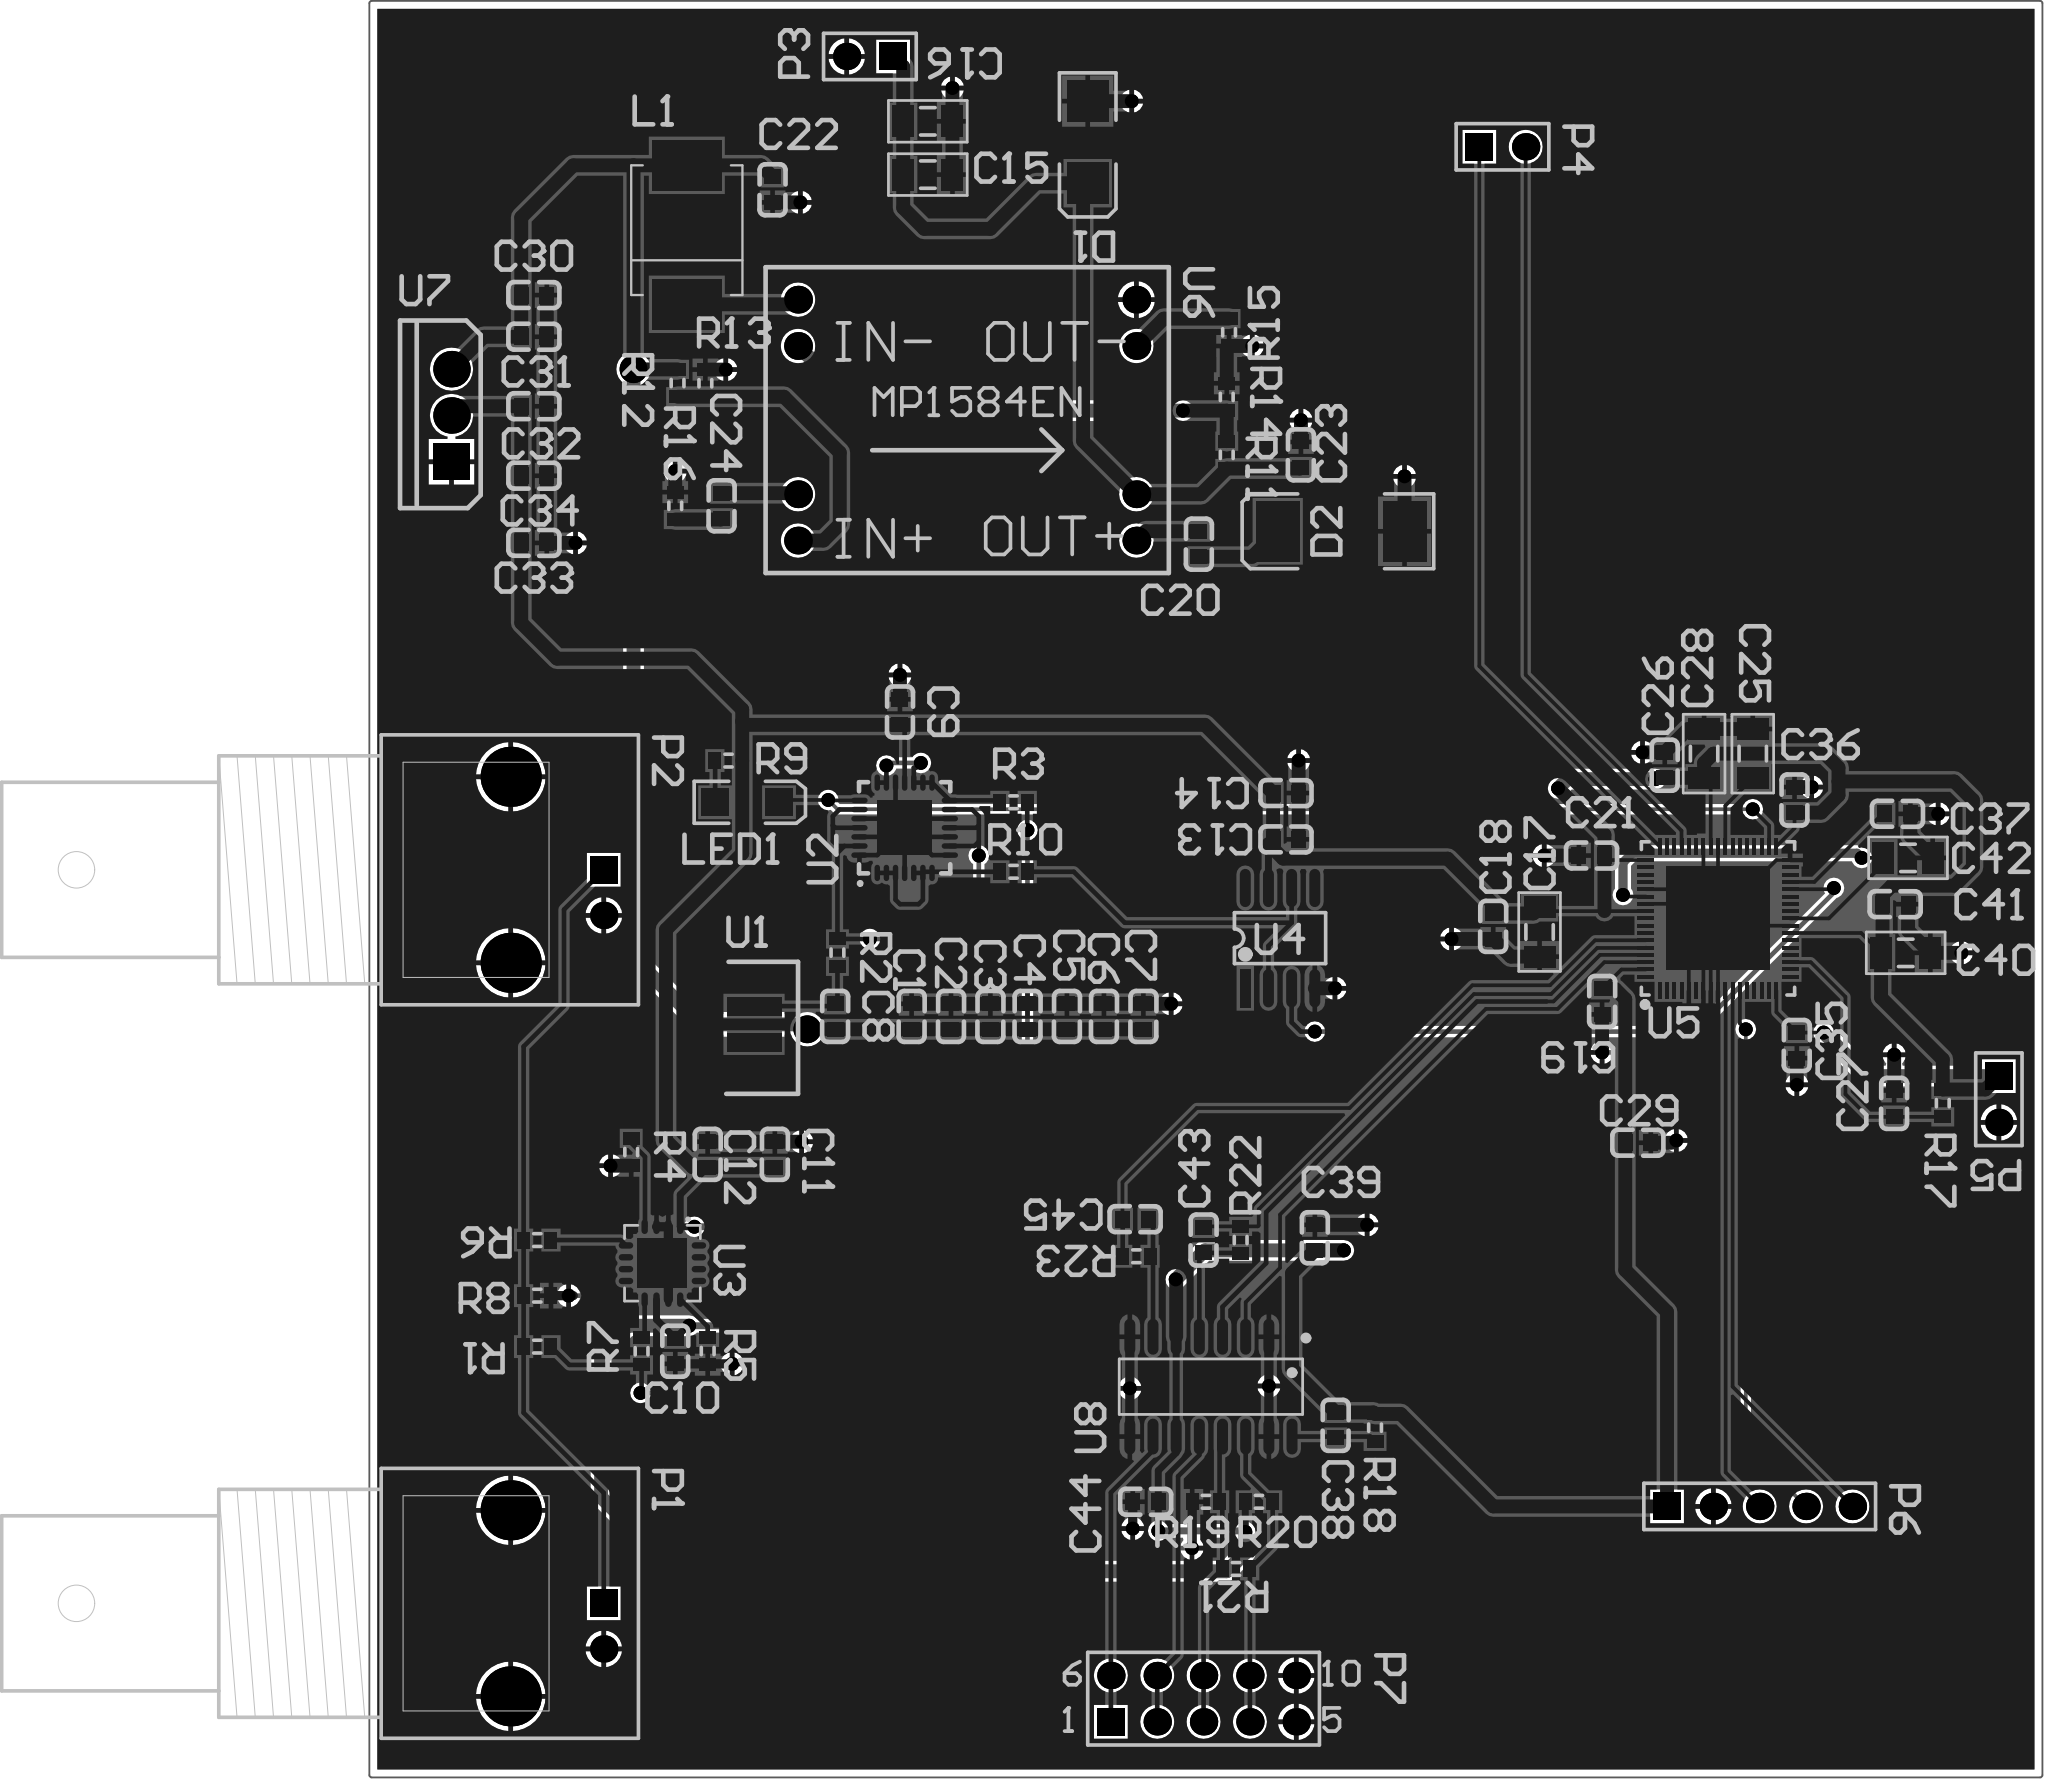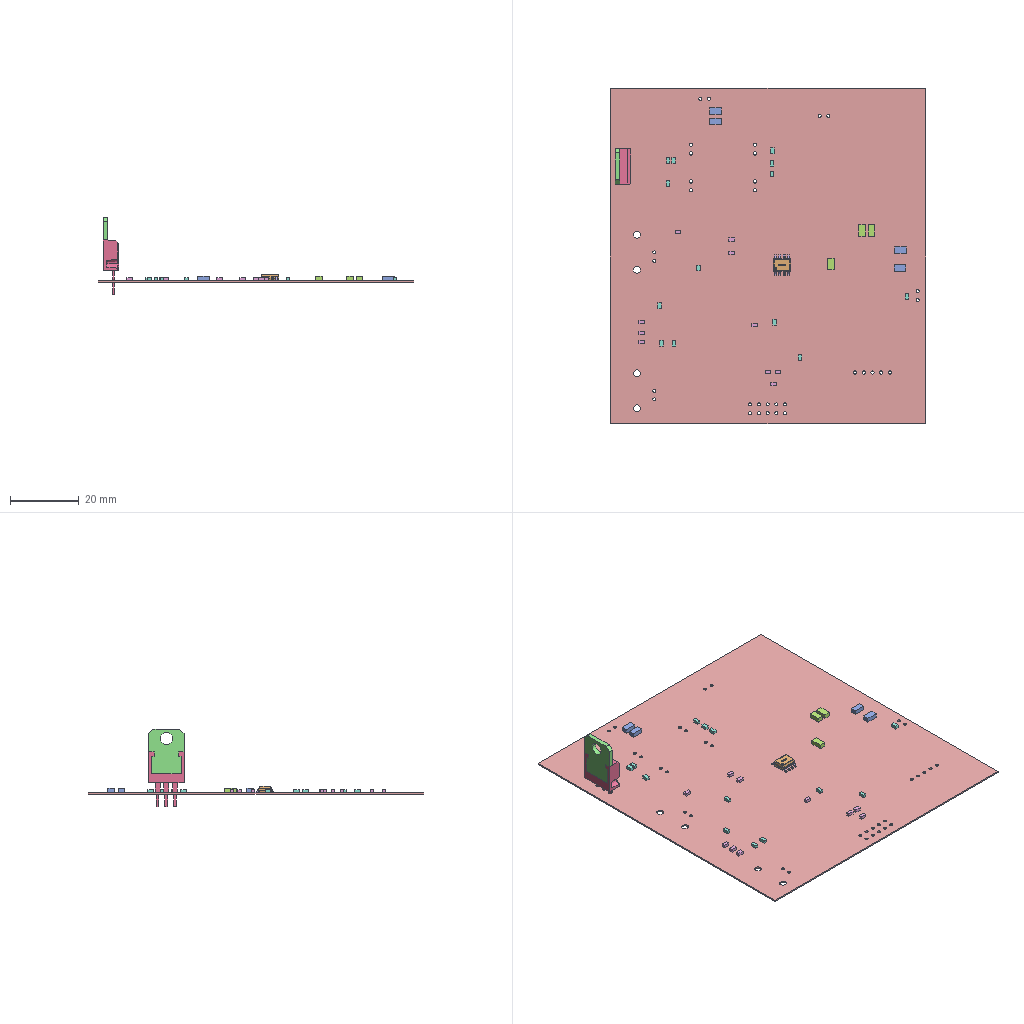Circuit board layout | Altium Designer | box 91.7 x 97.4 x 22.5 mm
Layer stack:
# Altium Designer layer stack of  (unit mm; dielectric type: 0 none, 1 core, 2 prepreg, 3 surface material)
index,name,kind,layer,copper_thickness_mm,dielectric_type,dielectric_thickness_mm,dielectric_material,dielectric_constant
0,Top Paste,other,,,,,,
1,Top Overlay,other,,,,,,
2,Top Solder,dielectric,,,3,0.0102,Solder Resist,3.5
3,Top Layer,copper,Top Layer,0.0356,,,,
4,Dielectric 1,dielectric,,,0,0.32,FR-4,4.8
5,Bottom Layer,copper,Bottom Layer,0.0356,,,,
6,Bottom Solder,dielectric,,,3,0.0102,Solder Resist,3.5
7,Bottom Overlay,other,,,,,,
8,Bottom Paste,other,,,,,,
# drill layer pairs: low layer,high layer
drill_pair,Top Layer,Bottom Layer
Part placement:
Designator,Comment,Layer,Footprint,Center-X(mm),Center-Y(mm),Rotation
C1,10UF,TopLayer,C0603,54.991,71.436,270
C2,10UF,TopLayer,C0603,57.15,71.436,270
C3,10UF,TopLayer,C0603,59.309,71.436,270
C4,10UF,TopLayer,C0603,61.344,71.436,270
C5,10UF,TopLayer,C0603,63.503,71.436,270
C6,0.1UF,TopLayer,C0603,65.532,71.436,270
C7,10UF,TopLayer,C0603,67.694,71.436,270
C8,100PF,TopLayer,C0603,50.797,71.436,270
C9,10UF,TopLayer,C0603,54.353,88.13,270
C10,0.1UF,TopLayer,C0603,42.04,53.094,90
C11,0.1UF,TopLayer,C0603,47.495,63.873,270
C12,10UF,TopLayer,C0603,43.812,63.873,270
C13,0.1UF,TopLayer,C0603,75.503,81.153,180
C14,10UF,TopLayer,C0603,75.503,83.693,180
C15,10UF/50V,TopLayer,C1206,55.88,117.602,180
C16,10UF/50V,TopLayer,C1206,55.88,120.523,180
C17,1UF/16V,TopLayer,C1206,89.408,76.073,90
C18,0.1UF,TopLayer,C0603,86.868,76.389,90
C19,0.1UF,TopLayer,C0603,92.834,72.255,270
C20,0.1UF,TopLayer,C0603,70.739,97.347,90
C21,0.1UF,TopLayer,C0603,92.264,80.264,0
C22,22UF,TopLayer,C0603,47.371,116.778,90
C23,10UF,TopLayer,C0603,76.33,102.243,90
C24,150PF,TopLayer,C0603,44.574,99.433,270
C25,1UF/16V,TopLayer,C1206,101.092,85.852,270
C26,0.1UF,TopLayer,C0603,96.269,85.225,90
C27,10nf,TopLayer,C0603,108.842,66.683,90
C28,1UF/16V,TopLayer,C1206,98.425,85.852,90
C29,0.1UF,TopLayer,C0603,94.804,64.516,360
C30,10UF,TopLayer,C0603,34.298,110.995,360
C31,0.1UF,TopLayer,C0603,34.298,108.709,360
C32,10UF,TopLayer,C0603,34.298,104.899,360
C33,1UF,TopLayer,C0603,34.298,97.406,360
C34,0.1UF,TopLayer,C0603,34.298,101.089,360
C35,0.1UF,TopLayer,C0603,103.508,69.858,90
C36,0.1UF,TopLayer,C0603,103.381,83.32,90
C37,0.1UF,TopLayer,C0603,109.031,82.55,360
C38,12PF,TopLayer,C0603,78.235,49.03,90
C39,0.1UF,TopLayer,C0603,77.092,59.317,90
C40,1UF/16V,TopLayer,C1206,109.474,74.93,360
C41,0.1UF,TopLayer,C0603,108.904,77.597,360
C42,1UF/16V,TopLayer,C1206,109.601,80.137,360
C43,12PF,TopLayer,C0603,70.99,59.174,270
C44,01.UF,TopLayer,C0603,67.81,44.834,180
C45,12PF,TopLayer,C0603,67.248,60.325,360
D1,D Schottky,TopLayer,SMB,64.643,119.38,270
D2,S320,TopLayer,SMC,78.532,98.044,180
L1,22UH,TopLayer,DIODE_SMC,42.672,114.3,90
LED1,LED2,TopLayer,3.2X1.6X1.1,45.974,83.185,360
P1,BNC,TopLayer,BNC_RA_CON,35.57,39.263,360
P2,BNC,TopLayer,BNC_RA_CON,35.57,79.482,360
P3,Header 2,TopLayer,HDR1X2,52.705,124.079,180
P4,Header 2,TopLayer,HDR1X2,87.376,119.126,360
P5,Header 2,TopLayer,HDR1X2,114.581,66.902,270
P6,Header 5,TopLayer,HDR1X5,101.473,44.577,360
P7,Header 5X2A,TopLayer,HDR2X5_CEN,70.993,34.036,360
R1,N/A,TopLayer,J1-0603,34.477,53.34,180
R2,0.1,TopLayer,J1-0603,50.927,74.942,270
R3,33,TopLayer,J1-0603,60.579,83.185,0
R4,4.7K,TopLayer,J1-0603,39.624,64.008,270
R5,4.7K,TopLayer,J1-0603,43.815,53.098,90
R6,33,TopLayer,J1-0603,34.477,59.182,180
R7,0,TopLayer,J1-0603,40.192,53.086,90
R8,510,TopLayer,J1-0603,34.477,56.134,360
R9,10K,TopLayer,J1-0603,44.958,85.471,0
R10,33,TopLayer,J1-0603,60.579,79.375,360
R11,100K,TopLayer,J1-0603,72.263,102.235,270
R12,300K,TopLayer,J1-0603,42.164,106.172,270
R13,39K,TopLayer,J1-0603,43.688,106.16,90
R14,25K,TopLayer,J1-0603,72.263,105.41,270
R15,100K,TopLayer,J1-0603,72.39,108.954,90
R16,100K,TopLayer,J1-0603,42.037,99.441,270
R17,10K,TopLayer,J1-0603,111.506,66.687,90
R18,820,TopLayer,J1-0603,80.391,48.895,270
R19,510,TopLayer,J1-0603,71.12,44.831,360
R20,510,TopLayer,J1-0603,74.029,44.831,360
R21,120,TopLayer,J1-0603,72.771,41.148,180
R22,10K,TopLayer,J1-0603,73.025,59.182,90
R23,820,TopLayer,J1-0603,67.31,58.293,360
U1,Laser diode,TopLayer,激光二极管,46.355,71.009,90
U2,IC-HG,TopLayer,QFN28-5X5,54.61,81.788,90
U3,ISL55111IRZ-T,TopLayer,QFN-16_L4.0-W4.0-P0.65-BL-EP2.6,41.335,57.912,180
U4,OPA335AIDRG4,TopLayer,SOP8,75.184,75.736,90
U5,CY8C3245LTI-163,TopLayer,QFN-68_L8.0-W8.0-P0.40-TL-EP5.7,99.187,76.818,90
U7,LM317,TopLayer,TO220A,29.774,104.394,90
U8,IL3122-3E,TopLayer,SOIC-16_L9.9-W3.9-P1.27-LS6.0-BL,71.396,51.143,180
U6,MP1584ENZ,TopLayer,MP1548EN,58.038,104.14,360
Pad and via stacks:
# Altium Designer via and pad stacks of  (unit mm). Each distinct definition once, with the count of objects using it.
# via: kind,start_layer,end_layer,hole_mm,diameter_mm,mode(0 simple;1 top-mid-bottom;2 full stack),diameter_per_layer,count,example_net
# pad: kind,layer,hole_mm,hole_type(0 round;1 square;2 slot),plating,top_size,top_shape(1 round;2 rect;3 octagon;9 rounded rect),mid_size,bottom_size,mode,footprint,size_per_layer,count,example
pad,Top Layer,0,0,plated,0.8x0.9,2,0.8x0.9,0.8x0.9,0,C0603,,76,C45.2
pad,Top Layer,0,0,plated,0.9x0.7,2,0.9x0.7,0.9x0.7,0,J1-0603,,46,R23.2
pad,Top Layer,0,0,plated,1.7x1.2,2,1.7x1.2,1.7x1.2,0,C1206,,14,C40.2
pad,Top Layer,0,0,plated,0.602x1.971,1,0.602x1.971,0.602x1.971,0,SOIC-16_L9.9-W3.9-P1.27-LS6.0-BL,,16,U8.9
pad,Top Layer,0,0,plated,2.794x3.81,2,2.794x3.81,2.794x3.81,0,DIODE_SMC,,2,L1.1
pad,Top Layer,0,0,plated,0.2x0.9,2,0.2x0.9,0.2x0.9,0,QFN-68_L8.0-W8.0-P0.40-TL-EP5.7,,34,U5.17
pad,Top Layer,0,0,plated,5.7x5.7,2,5.7x5.7,5.7x5.7,0,QFN-68_L8.0-W8.0-P0.40-TL-EP5.7,,1,U5.69
pad,Top Layer,0,0,plated,0.9x0.2,2,0.9x0.2,0.9x0.2,0,QFN-68_L8.0-W8.0-P0.40-TL-EP5.7,,34,U5.18
pad,Top Layer,0,0,plated,2.4x3.3,2,2.4x3.3,2.4x3.3,0,SMC,,2,D2.2
pad,Top Layer,0,0,plated,2.3x2.3,2,2.3x2.3,2.3x2.3,0,SMB,,2,D1.1
pad,Top Layer,0,0,plated,1.5x1.5,2,1.5x1.5,1.5x1.5,0,3.2X1.6X1.1,,2,LED1.2
pad,Top Layer,0,0,plated,0.6x2.1,2,0.6x2.1,0.6x2.1,0,SOP8,,1,U4.1
pad,Top Layer,0,0,plated,0.6x2.1,1,0.6x2.1,0.6x2.1,0,SOP8,,7,U4.2
pad,Top Layer,0,0,plated,0.35x0.8,1,0.35x0.8,0.35x0.8,0,QFN-16_L4.0-W4.0-P0.65-BL-EP2.6,,8,U3.1
pad,Top Layer,0,0,plated,0.8x0.35,1,0.8x0.35,0.8x0.35,0,QFN-16_L4.0-W4.0-P0.65-BL-EP2.6,,8,U3.5
pad,Top Layer,0,0,plated,2.7x2.7,2,2.7x2.7,2.7x2.7,0,QFN-16_L4.0-W4.0-P0.65-BL-EP2.6,,1,U3.17
pad,Top Layer,0,0,plated,3x3,2,3x3,3x3,0,QFN28-5X5,,1,U2.29
pad,Top Layer,0,0,plated,0.3x0.9,1,0.3x0.9,0.3x0.9,0,QFN28-5X5,,28,U2.2
pad,Top Layer,0,0,plated,1x3,2,1x3,1x3,0,\u00BC\u00A4\u00B9\u00E2\u00B6\u00FE\u00BC\u00AB\u00B9\u00DC,,2,U1.1
pad,Multi-Layer,0.9,0,plated,1.5x1.5,2,1.5x1.5,1.5x1.5,0,HDR2X5_CEN,,1,P7.1
pad,Multi-Layer,0.9,0,plated,1.5x1.5,1,1.5x1.5,1.5x1.5,0,HDR2X5_CEN,,9,P7.2
pad,Multi-Layer,0.9,0,plated,1.5x1.5,2,1.5x1.5,1.5x1.5,0,HDR1X5,,1,P6.1
pad,Multi-Layer,0.9,0,plated,1.5x1.5,1,1.5x1.5,1.5x1.5,0,HDR1X5,,4,P6.2
pad,Multi-Layer,1.1,0,plated,2x2,2,2x2,2x2,0,TO220A,,1,U7.1
pad,Multi-Layer,1.1,0,plated,2x2,1,2x2,2x2,0,TO220A,,2,U7.3
pad,Multi-Layer,0.9,0,plated,1.5x1.5,1,1.5x1.5,1.5x1.5,0,HDR1X2,,3,P5.2
pad,Multi-Layer,0.9,0,plated,1.5x1.5,2,1.5x1.5,1.5x1.5,0,HDR1X2,,3,P5.1
pad,Multi-Layer,0.9,0,plated,1.5x1.5,2,1.5x1.5,1.5x1.5,0,BNC_RA CON,,2,P2.1
pad,Multi-Layer,0.9,0,plated,1.5x1.5,1,1.5x1.5,1.5x1.5,0,BNC_RA CON,,2,P2.2
pad,Multi-Layer,2,0,plated,3.3x3.3,1,3.3x3.3,3.3x3.3,0,BNC_RA CON,,4,P2.2
pad,Multi-Layer,1,0,plated,1.524x1.524,1,1.524x1.524,1.524x1.524,0,MP1548EN,,8,U6.8
pad,Bottom Layer,0,0,plated,1x3,2,1x3,1x3,0,\u00BC\u00A4\u00B9\u00E2\u00B6\u00FE\u00BC\u00AB\u00B9\u00DC,,1,U1.2
via,Top Layer,Bottom Layer,0.762,1.524,0,,2,VDD8V
via,Top Layer,Bottom Layer,0.381,0.762,0,,62,NetP6_4
Copper pours:
name,layer,net,type(0 solid;1 hatched;2 none)
G,Bottom Layer,GND,0
G,Top Layer,GND,0
Design rules, without the lines most boards share:
# Altium Designer design rules of  (exported by Altium Designer, unit mm)
# columns: name | kind | enabled | priority | scope1 | scope2 | descriptor | typed fields (field=value)
Clearance | 0 | enabled | 1 | All | All | Clearance Constraint (Gap=7mil) (All),(All) | gap=0.1778
PlaneConnect | 6 | enabled | 1 | All | All | Power Plane Connect Rule(Relief Connect )(Expansion=20mil) (Conductor Width=10mil) (Air Gap=10mil) (Entries=4) (All) | relief_conductor_width=0.254 relief_entries=4 relief_expansion=0.508
PolygonConnect | 20 | enabled | 1 | All | All | Polygon Connect Rule(Relief Connect )(Conductor Width=10mil) (Relief Angle=90 Angle) (Entries=4) (Air Gap Width=10mil) (All),(All) | connect_style(0=relief,1=direct,2=none)=0 relief_conductor_width=0.254 relief_entries=4
Width | 2 | enabled | 1 | All | All | Width Constraint (Min=7mil) (Max=30mil) (Preferred=7mil) (All) |
RoutingVias | 11 | enabled | 1 | All | All | Routing Via (MinHoleWidth=28mil) (MaxHoleWidth=28mil) (PreferredHoleWidth=28mil) (MinWidth=50mil) (MaxWidth=50mil) (PreferedWidth=50mil) (All) | via_min_hole=0.7112 via_max_hole=0.7112 via_preferred_diameter=1.27 via_preferred_hole=0.7112
PasteMaskExpansion | 14 | enabled | 1 | All | All | Paste Mask Expansion (Expansion =0mil) (All) | expansion=0
SolderMaskExpansion | 13 | enabled | 1 | All | All | Solder Mask Expansion (Expansion =4mil) (All) | expansion=0.1016
DiffPairsRouting | 51 | enabled | 1 | All | All | Differential Pairs Uncoupled Length using the Gap Constraints (Min=10mil) (Max=10mil) (Prefered=10mil)  and Width Constraints (Min=15mil) (Max=15mil) (Prefered=15mil) (All) |
HoleToHoleClearance | 52 | enabled | 1 | All | All | Hole To Hole Clearance (Gap=10mil) (All),(All) | gap=0.254
MinimumSolderMaskSliver | 53 | enabled | 1 | All | All | Minimum Solder Mask Sliver (Gap=0mil) (All),(All) |
SilkToSolderMaskClearance | 54 | enabled | 1 | IsPad | All | Silk To Solder Mask (Clearance=0mil) (IsPad),(All) |
SilkToSilkClearance | 55 | enabled | 1 | All | All | Silk to Silk (Clearance=0mil) (All),(All) |
Classes set for this board:
# Altium Designer classes of  (member kind: 0 net, 1 component, 2 from-to, 3 pad, 4 layer, 5 differential pair, 6 design channel, 7 polygon, 8 structure, 9 xSignal)
# columns: class name | member kind | superclass | members
Sheet1 | 1 | no | C1; C2; C3; C4; C5; C6; C7; C8; C9; C10; C11; C12; C13; C14; C15; C16; C17; C18; C19; C20; C21; C22; C23; C24; C25; C26; C27; C28; C29; C30; C31; C32; C33; C34; C35; C36; C37; C38; C39; C40; C41; C42; C43; C44; C45; D1; D2; L1; LED1; P1; P2; P3; P4; P5; P6; P7; R1; R2; R3; R4; R5; R6; R7; R8; R9; R10; R11; R12; R13; R14; R15; R16; R17; R18; R19; R20; R21; R22; R23; U1; U2; U3; U4; U5; U6; U7; U8; U6;